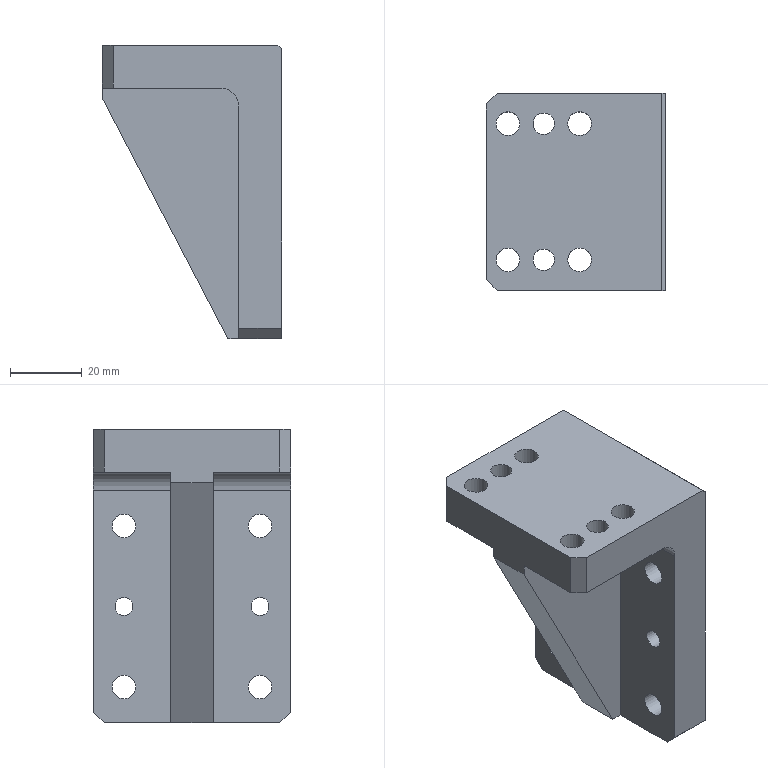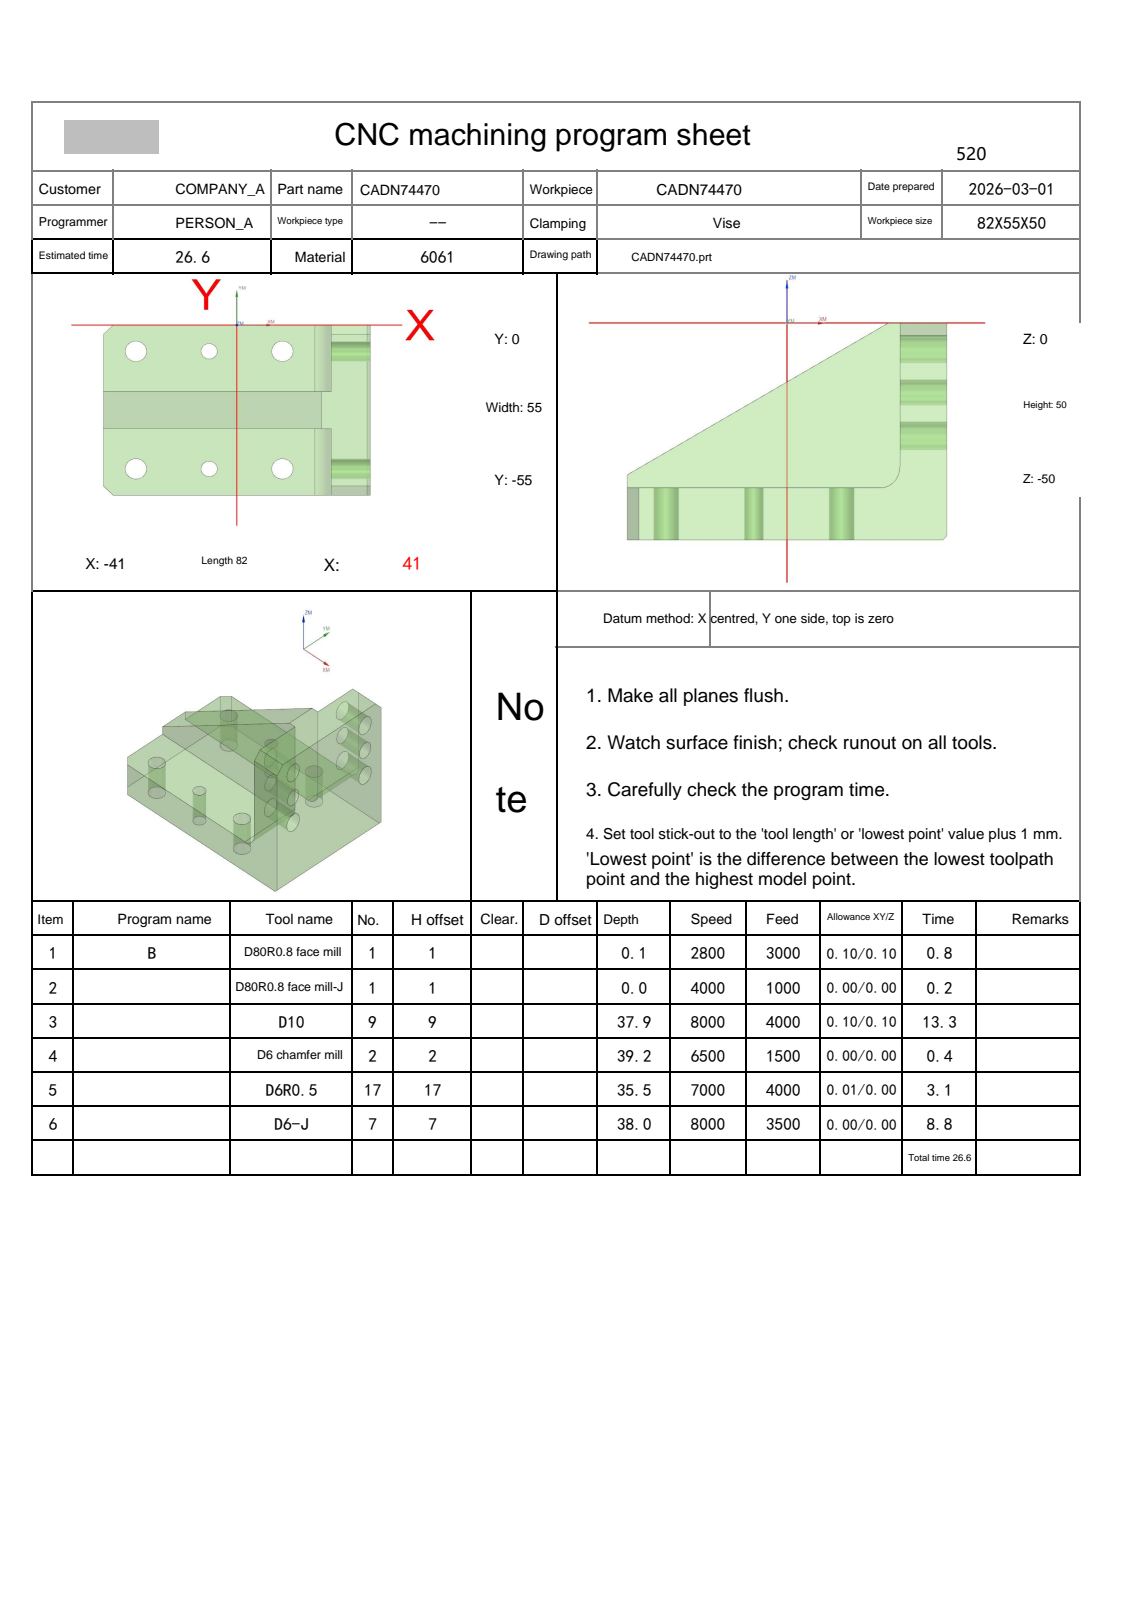NC program | NX | posted by the shop | part box 50 x 55 x 82 mm
Lines 8470 to 8651 of 26562:
N4 T02 M06
(D6 chamfer mill  D=6. R=0. H=02 ce=0.00 di=0.00)
G00 G90 G54 X28.01 Y-52.792 M03 S6500
G43 H02 Z50.
M08
Z.13
G01 Z-1.2 F1500.
G03 X28.085 Y-52.452 I-1.907 J.601
G01 X28.095 Y-52.398
X28.072 Y-52.349
X28.034 Y-52.259
X28. Y-52.
Y-34.5
X26.
X25.741 Y-34.466
X25.651 Y-34.428
Z2.8
G00 Z10.
Y-20.572
Z2.8
G01 Z-1.2
X25.741 Y-20.534
X26. Y-20.5
X28.
Y-3.
X28.034 Y-2.741
X28.072 Y-2.651
X28.095 Y-2.602
X28.085 Y-2.548
G03 X28.01 Y-2.208 I-1.983 J-.261
G01 Z.13
G00 Z10.
X41.99
Z.13
G01 Z-1.2
G03 X41.915 Y-2.548 I1.907 J-.601
G01 X41.905 Y-2.602
X41.928 Y-2.651
X41.966 Y-2.741
X42. Y-3.
Y-27.5
Y-52.
X41.966 Y-52.259
X41.928 Y-52.349
X41.905 Y-52.398
X41.915 Y-52.452
G03 X41.99 Y-52.792 I1.983 J.261
G01 Z.13
G00 Z10.
X-42.068 Y-18.472
Z-36.173
G01 Z-39.199
X-42.008 Y-18.386
X-42. Y-18.356
Y-3.
X-41.966 Y-2.741
X-41.866 Y-2.5
X-41.707 Y-2.293
X-38.707 Y.707
X-38.5 Y.866
X-38.259 Y.966
X-38. Y1.
X24.
X24.044 Y.996
X24.08 Y1.021
G03 X24.308 Y1.181 I-.8 J1.386
G01 Z-37.596
G00 Z10.
X11.892 Y-8.096
Z-37.747
G01 Z-39.199
G03 X11.718 Y-8.398 I1.638 J-1.147
G01 X11.692 Y-8.446
X11.7 Y-8.5
G03 X14. Y-10.8 I2.3 J0.0
X16.3 Y-8.5 I0.0 J2.3
X14. Y-6.2 I-2.3 J0.0
X11.7 Y-8.5 I0.0 J-2.3
G01 X11.692 Y-8.554
X11.718 Y-8.602
G03 X11.892 Y-8.904 I1.813 J.845
G01 Z-37.747
G00 Z10.
X-9.815 Y-8.093
Z-37.716
G01 Z-39.199
G03 X-9.984 Y-8.398 I1.658 J-1.118
G01 X-10.009 Y-8.446
X-10. Y-8.5
G03 X-8.5 Y-10. I1.5 J0.0
X-7. Y-8.5 I0.0 J1.5
X-8.5 Y-7. I-1.5 J0.0
X-10. Y-8.5 I0.0 J-1.5
G01 X-10.009 Y-8.554
X-9.984 Y-8.602
G03 X-9.815 Y-8.907 I1.827 J.813
G01 Z-37.716
G00 Z10.
X-33.108 Y-8.096
Z-37.747
G01 Z-39.199
G03 X-33.282 Y-8.398 I1.638 J-1.147
G01 X-33.308 Y-8.446
X-33.3 Y-8.5
G03 X-31. Y-10.8 I2.3 J0.0
X-28.7 Y-8.5 I0.0 J2.3
X-31. Y-6.2 I-2.3 J0.0
X-33.3 Y-8.5 I0.0 J-2.3
G01 X-33.308 Y-8.554
X-33.282 Y-8.602
G03 X-33.108 Y-8.904 I1.813 J.845
G01 Z-37.747
G00 Z10.
X24.308 Y-56.181
Z-37.596
G01 Z-39.199
G03 X24.08 Y-56.021 I-1.028 J-1.226
G01 X24.044 Y-55.996
X24. Y-56.
X-38.
X-38.259 Y-55.966
X-38.5 Y-55.866
X-38.707 Y-55.707
X-41.707 Y-52.707
X-41.866 Y-52.5
X-41.966 Y-52.259
X-42. Y-52.
Y-36.644
X-42.008 Y-36.614
X-42.068 Y-36.528
Z-36.173
G00 Z10.
X-33.108 Y-46.096
Z-37.747
G01 Z-39.199
G03 X-33.282 Y-46.398 I1.638 J-1.147
G01 X-33.308 Y-46.446
X-33.3 Y-46.5
G03 X-31. Y-48.8 I2.3 J0.0
X-28.7 Y-46.5 I0.0 J2.3
X-31. Y-44.2 I-2.3 J0.0
X-33.3 Y-46.5 I0.0 J-2.3
G01 X-33.308 Y-46.554
X-33.282 Y-46.602
G03 X-33.108 Y-46.904 I1.813 J.845
G01 Z-37.747
G00 Z10.
X-9.815 Y-46.093
Z-37.716
G01 Z-39.199
G03 X-9.984 Y-46.398 I1.658 J-1.118
G01 X-10.009 Y-46.446
X-10. Y-46.5
G03 X-8.5 Y-48. I1.5 J0.0
X-7. Y-46.5 I0.0 J1.5
X-8.5 Y-45. I-1.5 J0.0
X-10. Y-46.5 I0.0 J-1.5
G01 X-10.009 Y-46.554
X-9.984 Y-46.602
G03 X-9.815 Y-46.907 I1.827 J.813
G01 Z-37.716
G00 Z10.
X11.892 Y-46.096
Z-37.747
G01 Z-39.199
G03 X11.718 Y-46.398 I1.638 J-1.147
G01 X11.692 Y-46.446
X11.7 Y-46.5
G03 X14. Y-48.8 I2.3 J0.0
X16.3 Y-46.5 I0.0 J2.3
X14. Y-44.2 I-2.3 J0.0
X11.7 Y-46.5 I0.0 J-2.3
G01 X11.692 Y-46.554
X11.718 Y-46.602
G03 X11.892 Y-46.904 I1.813 J.845
G01 Z-37.747
G00 Z50.
G91 G28 Z0.0
M05
M09
G91 G28 Z0.0
M01